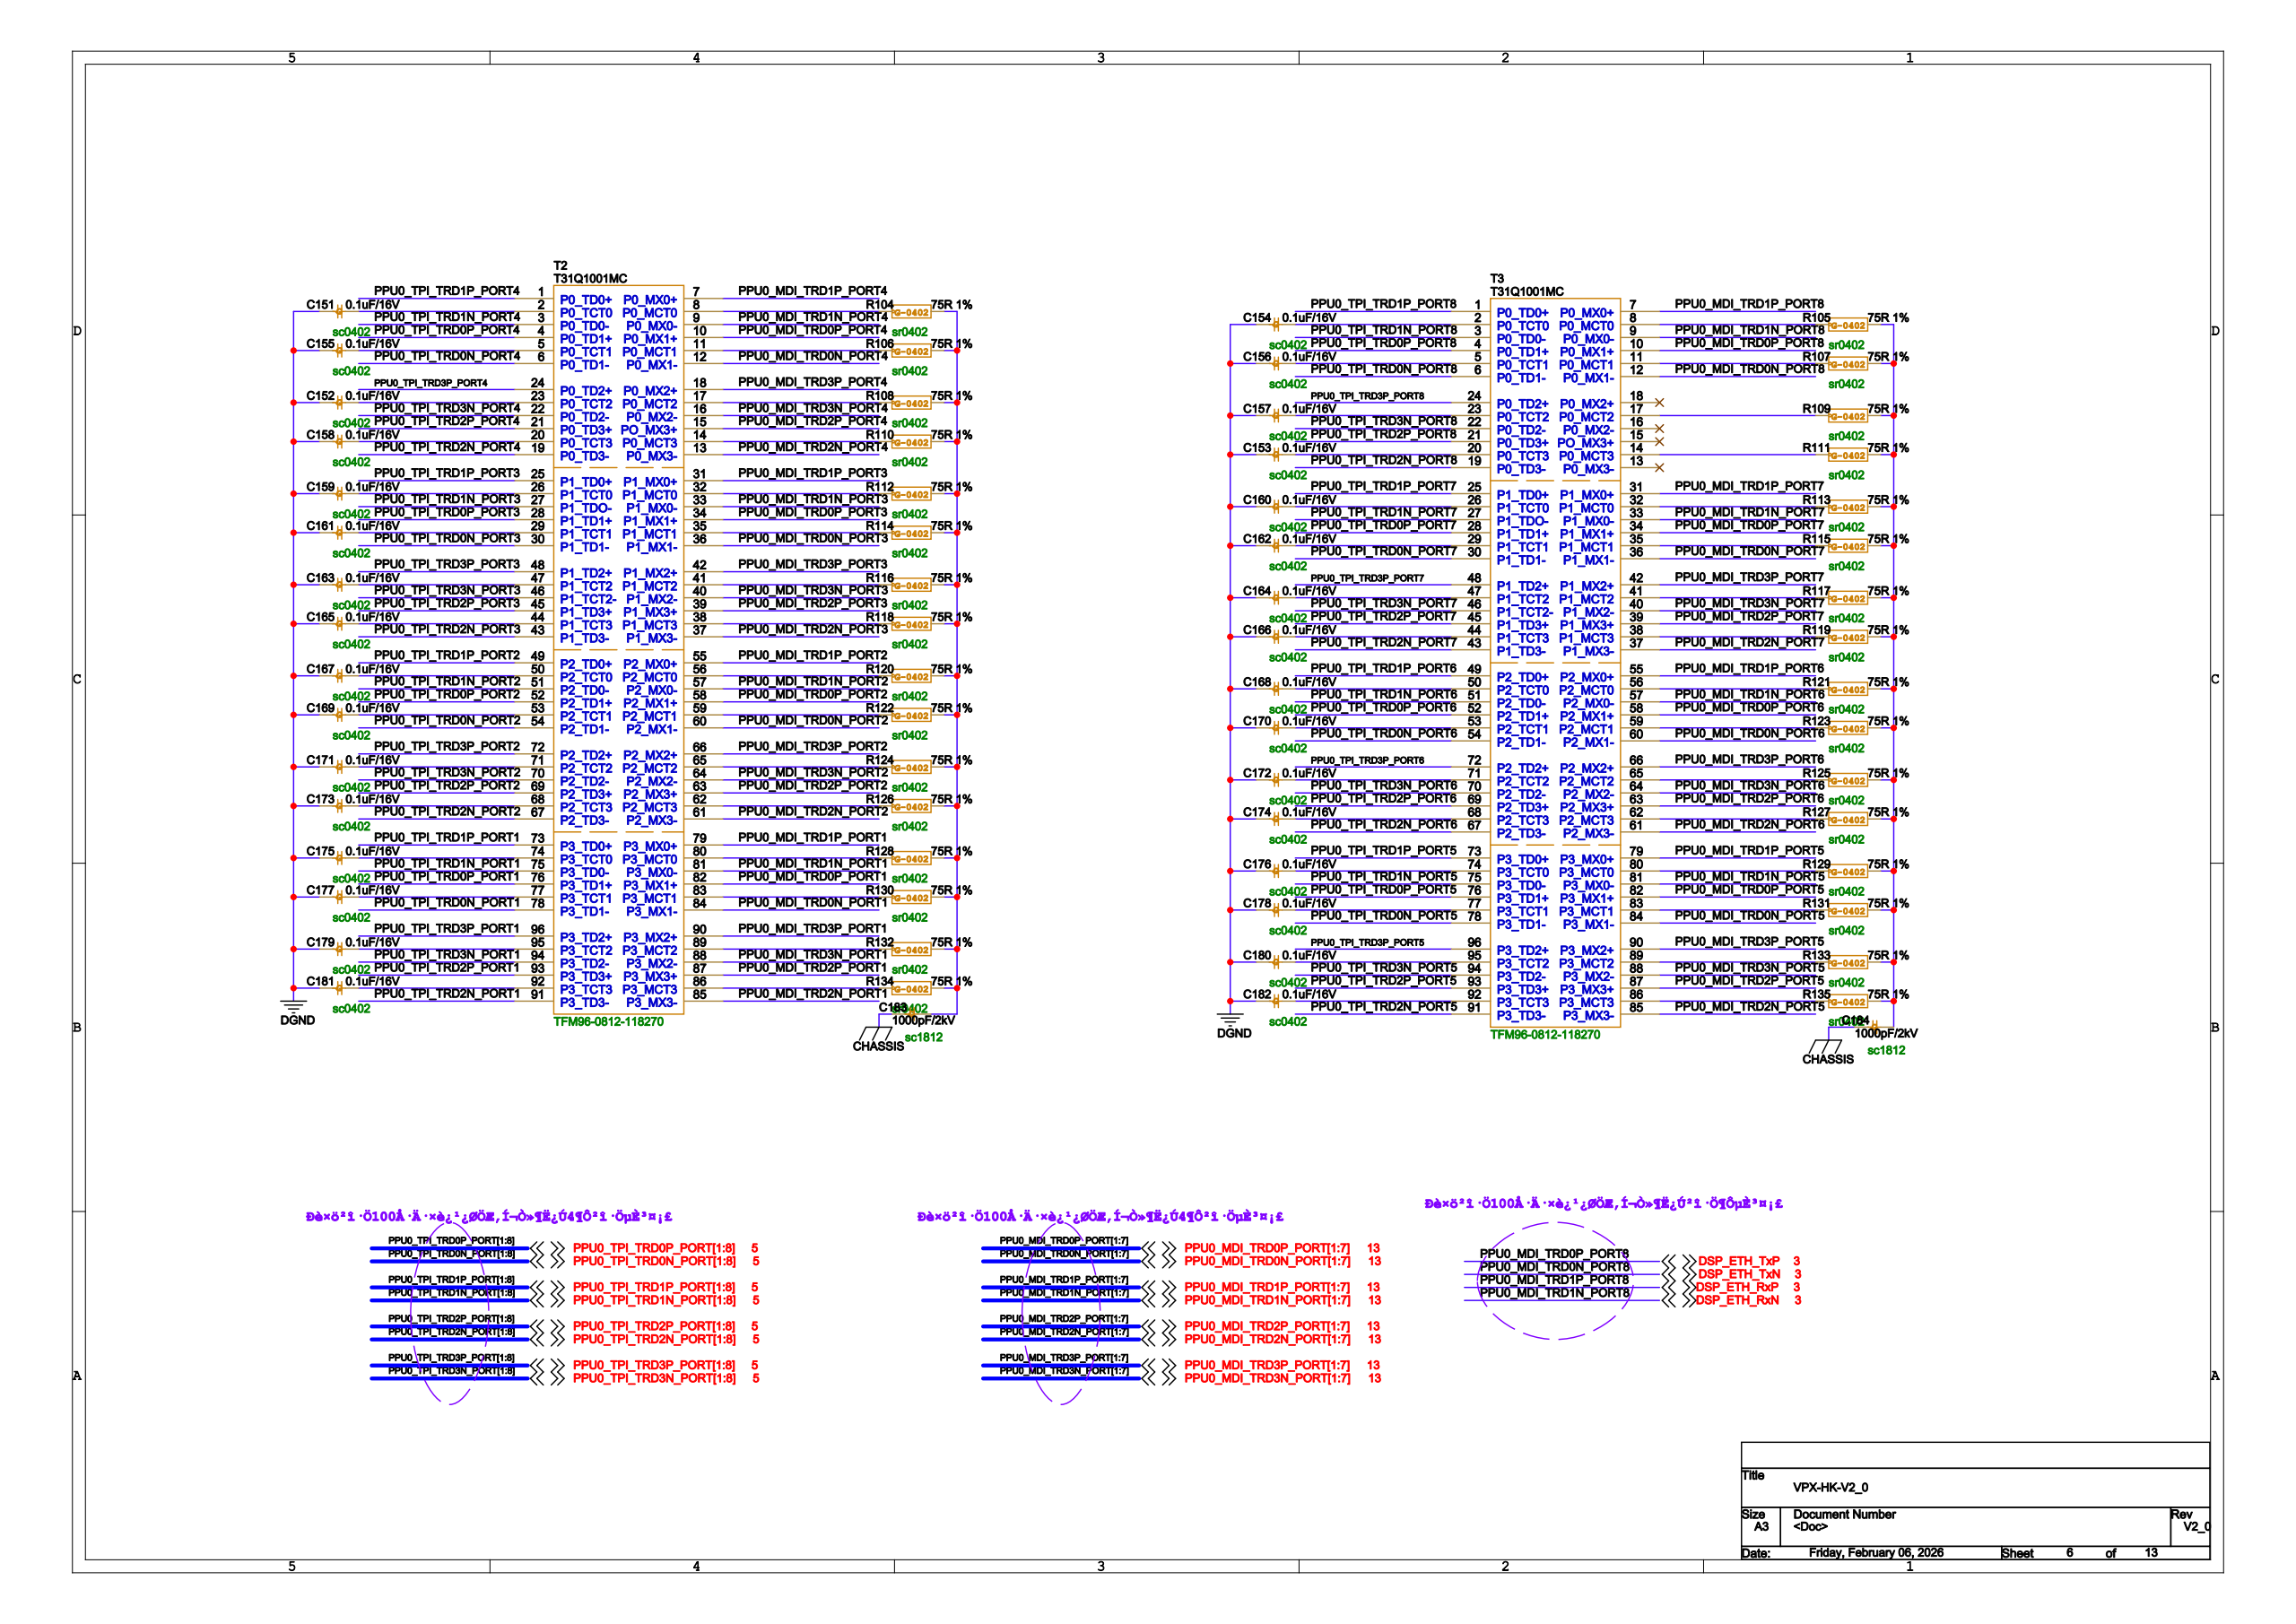Circuit board | Cadence Allegro | 598 parts | 541 nets | one sheet of the schematic
Parts on this sheet (reference | value | footprint):
C151 | 0.1uF/16V | SC0402
C152 | 0.1uF/16V | SC0402
C153 | 0.1uF/16V | SC0402
C154 | 0.1uF/16V | SC0402
C155 | 0.1uF/16V | SC0402
C156 | 0.1uF/16V | SC0402
C157 | 0.1uF/16V | SC0402
C158 | 0.1uF/16V | SC0402
C159 | 0.1uF/16V | SC0402
C160 | 0.1uF/16V | SC0402
C161 | 0.1uF/16V | SC0402
C162 | 0.1uF/16V | SC0402
C163 | 0.1uF/16V | SC0402
C164 | 0.1uF/16V | SC0402
C165 | 0.1uF/16V | SC0402
C166 | 0.1uF/16V | SC0402
C167 | 0.1uF/16V | SC0402
C168 | 0.1uF/16V | SC0402
C169 | 0.1uF/16V | SC0402
C170 | 0.1uF/16V | SC0402
C171 | 0.1uF/16V | SC0402
C172 | 0.1uF/16V | SC0402
C173 | 0.1uF/16V | SC0402
C174 | 0.1uF/16V | SC0402
C175 | 0.1uF/16V | SC0402
C176 | 0.1uF/16V | SC0402
C177 | 0.1uF/16V | SC0402
C178 | 0.1uF/16V | SC0402
C179 | 0.1uF/16V | SC0402
C180 | 0.1uF/16V | SC0402
C181 | 0.1uF/16V | SC0402
C182 | 0.1uF/16V | SC0402
C183 | 1000pF/2kV | SC1812
C184 | 1000pF/2kV | SC1812
R104 | 75R 1% | SR0402
R105 | 75R 1% | SR0402
R106 | 75R 1% | SR0402
R107 | 75R 1% | SR0402
R108 | 75R 1% | SR0402
R109 | 75R 1% | SR0402
R110 | 75R 1% | SR0402
R111 | 75R 1% | SR0402
R112 | 75R 1% | SR0402
R113 | 75R 1% | SR0402
R114 | 75R 1% | SR0402
R115 | 75R 1% | SR0402
R116 | 75R 1% | SR0402
R117 | 75R 1% | SR0402
R118 | 75R 1% | SR0402
R119 | 75R 1% | SR0402
R120 | 75R 1% | SR0402
R121 | 75R 1% | SR0402
R122 | 75R 1% | SR0402
R123 | 75R 1% | SR0402
R124 | 75R 1% | SR0402
R125 | 75R 1% | SR0402
R126 | 75R 1% | SR0402
R127 | 75R 1% | SR0402
R128 | 75R 1% | SR0402
R129 | 75R 1% | SR0402
R130 | 75R 1% | SR0402
R131 | 75R 1% | SR0402
R132 | 75R 1% | SR0402
R133 | 75R 1% | SR0402
R134 | 75R 1% | SR0402
R135 | 75R 1% | SR0402
T2 | T31Q1001MC | TFM96-0812-118270
T3 | T31Q1001MC | TFM96-0812-118270
Nets of these parts (net: part-pin ...):
DGND: C151-1 C152-1 C153-1 C154-1 C155-1 C156-1 C157-1 C158-1 C159-1 C160-1 C161-1 C162-1 C163-1 C164-1 C165-1 C166-1 C167-1 C168-1 C169-1 C170-1 C171-1 C172-1 C173-1 C174-1 C175-1 C176-1 C177-1 C178-1 C179-1 C180-1 C181-1 C182-1
CHASSIS: C183-1 C184-1
N32696417: C182-2 T3-92
N32692527: C151-2 T2-2
N32692641: C152-2 T2-23
N32695867: C153-2 T3-20
N32695737: C154-2 T3-2
N32692580: C155-2 T2-5
N32695770: C156-2 T3-5
N32695819: C157-2 T3-23
N32692717: C158-2 T2-20
N32692792: C159-2 T2-26
N32696400: C160-2 T3-26
N32692852: C161-2 T2-29
N32696368: C162-2 T3-29
N32692110: C163-2 T2-47
N32696454: C164-2 T3-47
N32692148: C165-2 T2-44
N32695699: C166-2 T3-44
N32692281: C167-2 T2-50
N32695717: C168-2 T3-50
N32692305: C169-2 T2-53
N32695752: C170-2 T3-53
N32692331: C171-2 T2-71
N32695797: C172-2 T3-71
N32692454: C173-2 T2-68
N32695847: C174-2 T3-68
N32692676: C175-2 T2-74
N32696026: C176-2 T3-74
N32692761: C177-2 T2-77
N32696113: C178-2 T3-77
N32692830: C179-2 T2-95
N32696346: C180-2 T3-95
N32692088: C181-2 T2-92
PPU0_MDI_TRD0P_PORT1: T2-82
PPU0_MDI_TRD0P_PORT2: T2-58
PPU0_MDI_TRD0P_PORT3: T2-34
PPU0_MDI_TRD0P_PORT4: T2-10
PPU0_MDI_TRD2P_PORT4: T2-15
PPU0_MDI_TRD0N_PORT1: T2-84
PPU0_MDI_TRD2P_PORT1: T2-87
PPU0_MDI_TRD0N_PORT2: T2-60
PPU0_MDI_TRD2P_PORT2: T2-63
PPU0_MDI_TRD0N_PORT3: T2-36
PPU0_MDI_TRD2P_PORT3: T2-39
PPU0_MDI_TRD0N_PORT4: T2-12
PPU0_MDI_TRD2N_PORT4: T2-13
PPU0_MDI_TRD2N_PORT1: T2-85
PPU0_MDI_TRD2N_PORT2: T2-61
PPU0_MDI_TRD2N_PORT3: T2-37
PPU0_MDI_TRD1P_PORT1: T2-79
PPU0_MDI_TRD1P_PORT2: T2-55
PPU0_MDI_TRD1P_PORT3: T2-31
PPU0_MDI_TRD1P_PORT4: T2-7
PPU0_MDI_TRD3P_PORT4: T2-18
PPU0_MDI_TRD1N_PORT1: T2-81
PPU0_MDI_TRD3P_PORT1: T2-90
PPU0_MDI_TRD1N_PORT2: T2-57
PPU0_MDI_TRD3P_PORT2: T2-66
PPU0_MDI_TRD1N_PORT3: T2-33
PPU0_MDI_TRD3P_PORT3: T2-42
PPU0_MDI_TRD1N_PORT4: T2-9
PPU0_MDI_TRD3N_PORT4: T2-16
PPU0_MDI_TRD3N_PORT1: T2-88
PPU0_MDI_TRD3N_PORT2: T2-64
PPU0_MDI_TRD3N_PORT3: T2-40
PPU0_MDI_TRD0P_PORT6: T3-58
PPU0_MDI_TRD0P_PORT5: T3-82
PPU0_MDI_TRD0P_PORT7: T3-34
PPU0_MDI_TRD2P_PORT7: T3-39
PPU0_MDI_TRD0N_PORT6: T3-60
PPU0_MDI_TRD2P_PORT6: T3-63
PPU0_MDI_TRD0N_PORT5: T3-84
PPU0_MDI_TRD2P_PORT5: T3-87
PPU0_MDI_TRD0N_PORT7: T3-36
PPU0_MDI_TRD2N_PORT7: T3-37
PPU0_MDI_TRD2N_PORT6: T3-61
PPU0_MDI_TRD2N_PORT5: T3-85
PPU0_MDI_TRD1P_PORT6: T3-55
PPU0_MDI_TRD1P_PORT5: T3-79
PPU0_MDI_TRD1P_PORT7: T3-31
PPU0_MDI_TRD3P_PORT7: T3-42
PPU0_MDI_TRD1N_PORT6: T3-57
PPU0_MDI_TRD3P_PORT6: T3-66
PPU0_MDI_TRD1N_PORT5: T3-81
PPU0_MDI_TRD3P_PORT5: T3-90
PPU0_MDI_TRD1N_PORT7: T3-33
PPU0_MDI_TRD3N_PORT7: T3-40
PPU0_MDI_TRD3N_PORT6: T3-64
PPU0_MDI_TRD3N_PORT5: T3-88
PPU0_TPI_TRD0N_PORT1: T2-78
PPU0_TPI_TRD0P_PORT1: T2-76
PPU0_TPI_TRD1N_PORT1: T2-75
PPU0_TPI_TRD1P_PORT1: T2-73
PPU0_TPI_TRD2N_PORT1: T2-91
PPU0_TPI_TRD2P_PORT1: T2-93
PPU0_TPI_TRD3N_PORT1: T2-94
PPU0_TPI_TRD3P_PORT1: T2-96
PPU0_TPI_TRD0N_PORT2: T2-54
PPU0_TPI_TRD0P_PORT2: T2-52
PPU0_TPI_TRD1N_PORT2: T2-51
PPU0_TPI_TRD1P_PORT2: T2-49
PPU0_TPI_TRD2N_PORT2: T2-67
PPU0_TPI_TRD2P_PORT2: T2-69
PPU0_TPI_TRD3N_PORT2: T2-70
PPU0_TPI_TRD3P_PORT2: T2-72
PPU0_TPI_TRD0N_PORT3: T2-30
PPU0_TPI_TRD0P_PORT3: T2-28
PPU0_TPI_TRD1N_PORT3: T2-27
PPU0_TPI_TRD1P_PORT3: T2-25
PPU0_TPI_TRD2N_PORT3: T2-43
PPU0_TPI_TRD2P_PORT3: T2-45
PPU0_TPI_TRD3N_PORT3: T2-46
PPU0_TPI_TRD3P_PORT3: T2-48
PPU0_TPI_TRD0N_PORT4: T2-6
PPU0_TPI_TRD0P_PORT4: T2-4
PPU0_TPI_TRD1N_PORT4: T2-3
PPU0_TPI_TRD1P_PORT4: T2-1
PPU0_TPI_TRD2N_PORT4: T2-19
PPU0_TPI_TRD2P_PORT4: T2-21
PPU0_TPI_TRD3N_PORT4: T2-22
PPU0_TPI_TRD3P_PORT4: T2-24
PPU0_TPI_TRD0N_PORT5: T3-78
PPU0_TPI_TRD0P_PORT5: T3-76
PPU0_TPI_TRD1N_PORT5: T3-75
PPU0_TPI_TRD1P_PORT5: T3-73
PPU0_TPI_TRD2N_PORT5: T3-91
PPU0_TPI_TRD2P_PORT5: T3-93
PPU0_TPI_TRD3N_PORT5: T3-94
PPU0_TPI_TRD3P_PORT5: T3-96
PPU0_TPI_TRD0N_PORT6: T3-54
PPU0_TPI_TRD0P_PORT6: T3-52
PPU0_TPI_TRD1N_PORT6: T3-51
PPU0_TPI_TRD1P_PORT6: T3-49
PPU0_TPI_TRD2N_PORT6: T3-67
PPU0_TPI_TRD2P_PORT6: T3-69
PPU0_TPI_TRD3N_PORT6: T3-70
PPU0_TPI_TRD3P_PORT6: T3-72
PPU0_TPI_TRD0N_PORT7: T3-30
PPU0_TPI_TRD0P_PORT7: T3-28
PPU0_TPI_TRD1N_PORT7: T3-27
PPU0_TPI_TRD1P_PORT7: T3-25
PPU0_TPI_TRD2N_PORT7: T3-43
PPU0_TPI_TRD2P_PORT7: T3-45
PPU0_TPI_TRD3N_PORT7: T3-46
PPU0_TPI_TRD3P_PORT7: T3-48
PPU0_TPI_TRD0N_PORT8: T3-6
PPU0_TPI_TRD0P_PORT8: T3-4
PPU0_TPI_TRD1N_PORT8: T3-3
PPU0_TPI_TRD1P_PORT8: T3-1
PPU0_TPI_TRD2N_PORT8: T3-19
PPU0_TPI_TRD2P_PORT8: T3-21
PPU0_TPI_TRD3N_PORT8: T3-22
PPU0_TPI_TRD3P_PORT8: T3-24
N32695709: C184-2 R105-2 R107-2 R109-2 R111-2 R113-2 R115-2 R117-2 R119-2 R121-2 R123-2 R125-2 R127-2 R129-2 R131-2 R133-2 R135-2
N32692080: C183-2 R104-2 R106-2 R108-2 R110-2 R112-2 R114-2 R116-2 R118-2 R120-2 R122-2 R124-2 R126-2 R128-2 R130-2 R132-2 R134-2
N32696428: R135-1 T3-86
N32692519: R104-1 T2-8
N32695745: R105-1 T3-8
N32692578: R106-1 T2-11
N32695781: R107-1 T3-11
N32692624: R108-1 T2-17
N32695824: R109-1 T3-17
N32692709: R110-1 T2-14
N32695875: R111-1 T3-14
N32692800: R112-1 T2-32
N32696408: R113-1 T3-32
N32692860: R114-1 T2-35
N32696388: R115-1 T3-35
N32692118: R116-1 T2-41
N32696459: R117-1 T3-41
N32692156: R118-1 T2-38
N32695707: R119-1 T3-38
N32692289: R120-1
N32695725: R121-1
N32692313: R122-1 T2-59
N32695763: R123-1 T3-59
N32692339: R124-1 T2-65
N32695802: R125-1 T3-65
N32692462: R126-1 T2-62
N32695855: R127-1 T3-62
N32692693: R128-1 T2-80
N32696034: R129-1 T3-80
N32692778: R130-1 T2-83
N32696130: R131-1 T3-83
N32692838: R132-1 T2-89
N32696360: R133-1 T3-89
N32692096: R134-1 T2-86